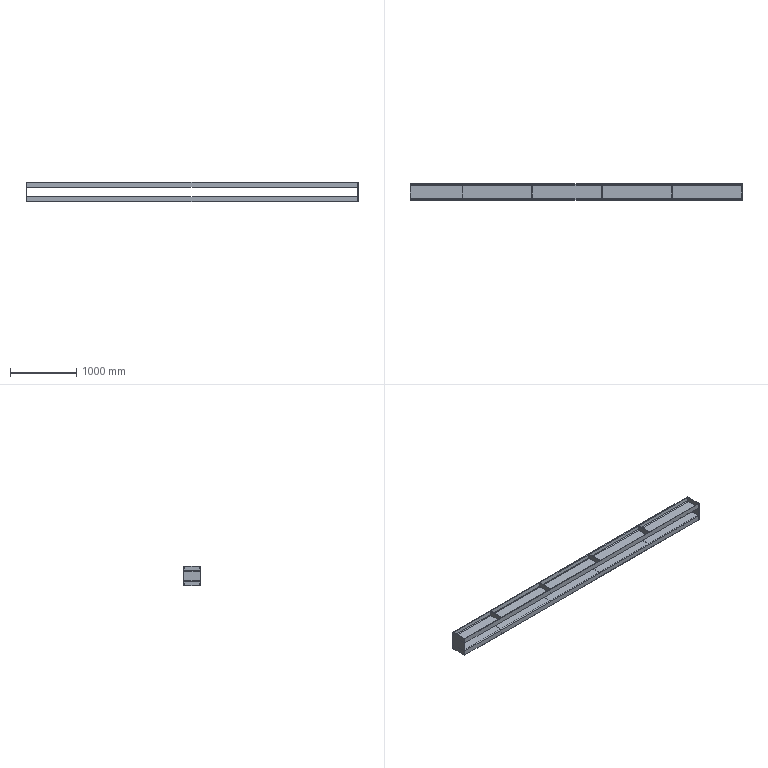Part | STEP file | Motor bracket lower channel steel_Default<As machined> | 12 solids | 120 faces | box 5000 x 250 x 300 mm | volume 37542692 mm3 | plane 80 | cylinder 40 | commonest cylinder face diameters 12 x20 24 x20